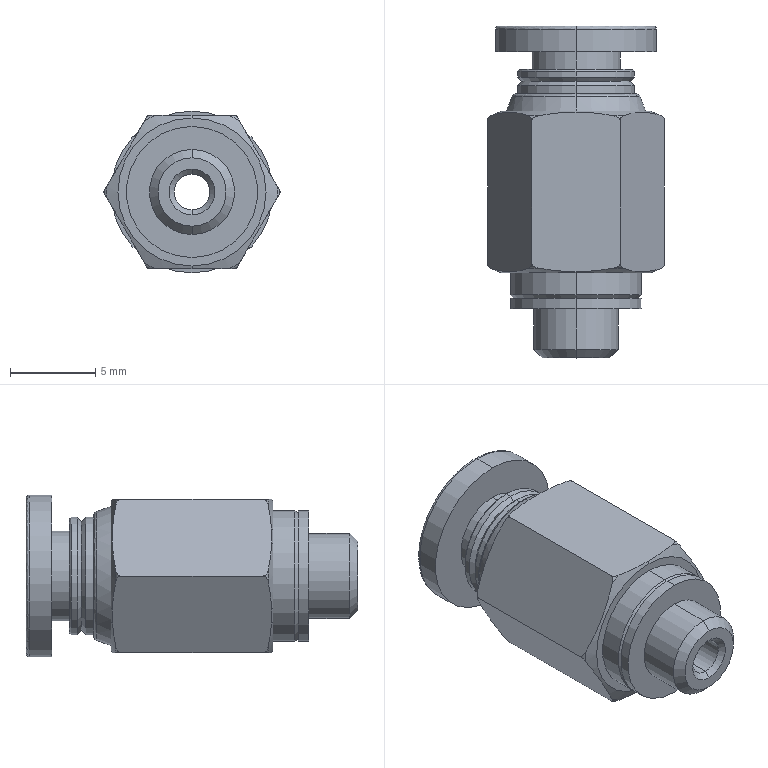Part | SolidWorks | features BaseBody 1 | 1 solid | 71 faces | box 10.392 x 19.5 x 9.5 mm | volume 848.842 mm3 | cone 20 | spline 18 | cylinder 18 | plane 15 | commonest cylinder face diameters 6.9 x4 7.7 x4 2.1 x2 4 x2 5 x2 5.26 x2